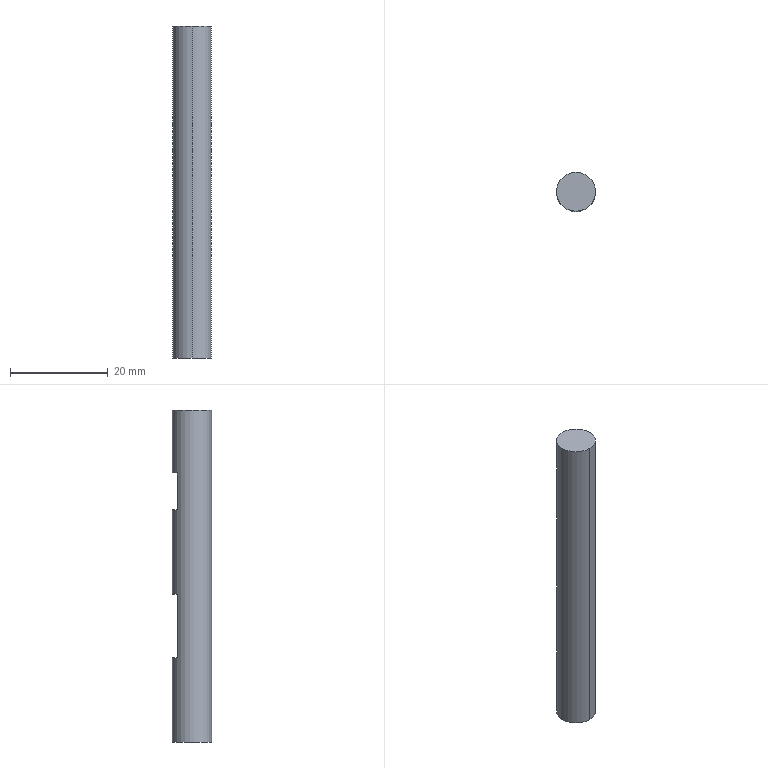Part | NX | 1 solid | 18 faces | box 8 x 8 x 68 mm | volume 3235 mm3 | plane 8 | cylinder 6 | cone 4 | commonest cylinder face diameters 3.3 x4 8 x2
STEP:
#1=CARTESIAN_POINT('',(-190.,200.7,-65.8));
#2=VERTEX_POINT('',#1);
#3=CARTESIAN_POINT('',(-190.,192.7,-65.8));
#4=VERTEX_POINT('',#3);
#5=CARTESIAN_POINT('',(-190.,196.7,-65.8));
#6=DIRECTION('',(0.,0.,1.));
#7=DIRECTION('',(0.,-1.,0.));
#8=AXIS2_PLACEMENT_3D('',#5,#6,#7);
#9=CIRCLE('',#8,4.);
#10=EDGE_CURVE('',#2,#4,#9,.T.);
#11=ORIENTED_EDGE('',*,*,#10,.T.);
#12=CARTESIAN_POINT('',(-190.,192.7,2.2));
#13=VERTEX_POINT('',#12);
#14=CARTESIAN_POINT('',(-190.,192.7,-55.8));
#15=DIRECTION('',(0.,0.,1.));
#16=VECTOR('',#15,1000.);
#17=LINE('',#14,#16);
#18=EDGE_CURVE('',#13,#4,#17,.F.);
#19=ORIENTED_EDGE('',*,*,#18,.F.);
#20=CARTESIAN_POINT('',(-190.,200.7,2.2));
#21=VERTEX_POINT('',#20);
#22=CARTESIAN_POINT('',(-190.,196.7,2.2));
#23=DIRECTION('',(0.,0.,1.));
#24=DIRECTION('',(0.,-1.,0.));
#25=AXIS2_PLACEMENT_3D('',#22,#23,#24);
#26=CIRCLE('',#25,4.);
#27=EDGE_CURVE('',#21,#13,#26,.T.);
#28=ORIENTED_EDGE('',*,*,#27,.F.);
#29=CARTESIAN_POINT('',(-190.,200.7,-10.7));
#30=VERTEX_POINT('',#29);
#31=CARTESIAN_POINT('',(-190.,200.7,-55.8));
#32=DIRECTION('',(0.,0.,1.));
#33=VECTOR('',#32,1000.);
#34=LINE('',#31,#33);
#35=EDGE_CURVE('',#30,#21,#34,.T.);
#36=ORIENTED_EDGE('',*,*,#35,.F.);
#37=CARTESIAN_POINT('',(-192.646,199.7,-10.7));
#38=VERTEX_POINT('',#37);
#39=CARTESIAN_POINT('',(-190.,196.7,-10.7));
#40=DIRECTION('',(0.,0.,1.));
#41=DIRECTION('',(0.,-1.,0.));
#42=AXIS2_PLACEMENT_3D('',#39,#40,#41);
#43=CIRCLE('',#42,4.);
#44=EDGE_CURVE('',#30,#38,#43,.T.);
#45=ORIENTED_EDGE('',*,*,#44,.T.);
#46=CARTESIAN_POINT('',(-192.646,199.7,-18.2));
#47=VERTEX_POINT('',#46);
#48=CARTESIAN_POINT('',(-192.646,199.7,-55.8));
#49=DIRECTION('',(0.,0.,1.));
#50=VECTOR('',#49,1000.);
#51=LINE('',#48,#50);
#52=EDGE_CURVE('',#47,#38,#51,.T.);
#53=ORIENTED_EDGE('',*,*,#52,.F.);
#54=CARTESIAN_POINT('',(-190.,200.7,-18.2));
#55=VERTEX_POINT('',#54);
#56=CARTESIAN_POINT('',(-190.,196.7,-18.2));
#57=DIRECTION('',(0.,0.,1.));
#58=DIRECTION('',(0.,-1.,0.));
#59=AXIS2_PLACEMENT_3D('',#56,#57,#58);
#60=CIRCLE('',#59,4.);
#61=EDGE_CURVE('',#55,#47,#60,.T.);
#62=ORIENTED_EDGE('',*,*,#61,.F.);
#63=CARTESIAN_POINT('',(-190.,200.7,-35.5));
#64=VERTEX_POINT('',#63);
#65=CARTESIAN_POINT('',(-190.,200.7,-55.8));
#66=DIRECTION('',(0.,0.,1.));
#67=VECTOR('',#66,1000.);
#68=LINE('',#65,#67);
#69=EDGE_CURVE('',#55,#64,#68,.F.);
#70=ORIENTED_EDGE('',*,*,#69,.T.);
#71=CARTESIAN_POINT('',(-192.646,199.7,-35.5));
#72=VERTEX_POINT('',#71);
#73=CARTESIAN_POINT('',(-190.,196.7,-35.5));
#74=DIRECTION('',(0.,0.,1.));
#75=DIRECTION('',(0.,-1.,0.));
#76=AXIS2_PLACEMENT_3D('',#73,#74,#75);
#77=CIRCLE('',#76,4.);
#78=EDGE_CURVE('',#64,#72,#77,.T.);
#79=ORIENTED_EDGE('',*,*,#78,.T.);
#80=CARTESIAN_POINT('',(-192.646,199.7,-48.5));
#81=VERTEX_POINT('',#80);
#82=CARTESIAN_POINT('',(-192.646,199.7,-55.8));
#83=DIRECTION('',(0.,0.,1.));
#84=VECTOR('',#83,1000.);
#85=LINE('',#82,#84);
#86=EDGE_CURVE('',#81,#72,#85,.T.);
#87=ORIENTED_EDGE('',*,*,#86,.F.);
#88=CARTESIAN_POINT('',(-190.,200.7,-48.5));
#89=VERTEX_POINT('',#88);
#90=CARTESIAN_POINT('',(-190.,196.7,-48.5));
#91=DIRECTION('',(0.,0.,1.));
#92=DIRECTION('',(0.,-1.,0.));
#93=AXIS2_PLACEMENT_3D('',#90,#91,#92);
#94=CIRCLE('',#93,4.);
#95=EDGE_CURVE('',#89,#81,#94,.T.);
#96=ORIENTED_EDGE('',*,*,#95,.F.);
#97=CARTESIAN_POINT('',(-190.,200.7,-55.8));
#98=DIRECTION('',(0.,0.,1.));
#99=VECTOR('',#98,1000.);
#100=LINE('',#97,#99);
#101=EDGE_CURVE('',#2,#89,#100,.T.);
#102=ORIENTED_EDGE('',*,*,#101,.F.);
#103=EDGE_LOOP('',(#11,#19,#28,#36,#45,#53,#62,#70,#79,#87,#96,#102));
#104=FACE_BOUND('',#103,.T.);
#105=CARTESIAN_POINT('',(-190.,196.7,-55.8));
#106=DIRECTION('',(0.,0.,1.));
#107=DIRECTION('',(0.,-1.,0.));
#108=AXIS2_PLACEMENT_3D('',#105,#106,#107);
#109=CYLINDRICAL_SURFACE('',#108,4.);
#110=ADVANCED_FACE('',(#104),#109,.T.);
#111=ORIENTED_EDGE('',*,*,#10,.F.);
#112=CARTESIAN_POINT('',(-190.,196.7,-65.8));
#113=DIRECTION('',(0.,0.,1.));
#114=DIRECTION('',(0.,-1.,0.));
#115=AXIS2_PLACEMENT_3D('',#112,#113,#114);
#116=CIRCLE('',#115,4.);
#117=EDGE_CURVE('',#4,#2,#116,.T.);
#118=ORIENTED_EDGE('',*,*,#117,.F.);
#119=EDGE_LOOP('',(#111,#118));
#120=FACE_BOUND('',#119,.T.);
#121=CARTESIAN_POINT('',(-187.685,196.7,-65.8));
#122=VERTEX_POINT('',#121);
#123=CARTESIAN_POINT('',(-192.315,196.7,-65.8));
#124=VERTEX_POINT('',#123);
#125=CARTESIAN_POINT('',(-190.,196.7,-65.8));
#126=DIRECTION('',(0.,0.,-1.));
#127=DIRECTION('',(-1.,0.,0.));
#128=AXIS2_PLACEMENT_3D('',#125,#126,#127);
#129=CIRCLE('',#128,2.315);
#130=EDGE_CURVE('',#122,#124,#129,.T.);
#131=ORIENTED_EDGE('',*,*,#130,.F.);
#132=CARTESIAN_POINT('',(-190.,196.7,-65.8));
#133=DIRECTION('',(0.,0.,-1.));
#134=DIRECTION('',(-1.,0.,0.));
#135=AXIS2_PLACEMENT_3D('',#132,#133,#134);
#136=CIRCLE('',#135,2.315);
#137=EDGE_CURVE('',#124,#122,#136,.T.);
#138=ORIENTED_EDGE('',*,*,#137,.F.);
#139=EDGE_LOOP('',(#131,#138));
#140=FACE_BOUND('',#139,.T.);
#141=CARTESIAN_POINT('',(-181.498,197.784,-65.8));
#142=DIRECTION('',(0.,0.,-1.));
#143=DIRECTION('',(-1.,0.,0.));
#144=AXIS2_PLACEMENT_3D('',#141,#142,#143);
#145=PLANE('',#144);
#146=ADVANCED_FACE('',(#120,#140),#145,.T.);
#147=ORIENTED_EDGE('',*,*,#27,.T.);
#148=CARTESIAN_POINT('',(-190.,196.7,2.2));
#149=DIRECTION('',(0.,0.,1.));
#150=DIRECTION('',(0.,-1.,0.));
#151=AXIS2_PLACEMENT_3D('',#148,#149,#150);
#152=CIRCLE('',#151,4.);
#153=EDGE_CURVE('',#13,#21,#152,.T.);
#154=ORIENTED_EDGE('',*,*,#153,.T.);
#155=EDGE_LOOP('',(#147,#154));
#156=FACE_BOUND('',#155,.T.);
#157=CARTESIAN_POINT('',(-181.498,197.784,2.2));
#158=DIRECTION('',(0.,0.,-1.));
#159=DIRECTION('',(-1.,0.,0.));
#160=AXIS2_PLACEMENT_3D('',#157,#158,#159);
#161=PLANE('',#160);
#162=ADVANCED_FACE('',(#156),#161,.F.);
#163=CARTESIAN_POINT('',(-187.354,199.7,-48.5));
#164=VERTEX_POINT('',#163);
#165=CARTESIAN_POINT('',(-187.354,199.7,-35.5));
#166=VERTEX_POINT('',#165);
#167=CARTESIAN_POINT('',(-187.354,199.7,-55.8));
#168=DIRECTION('',(0.,0.,1.));
#169=VECTOR('',#168,1000.);
#170=LINE('',#167,#169);
#171=EDGE_CURVE('',#164,#166,#170,.T.);
#172=ORIENTED_EDGE('',*,*,#171,.F.);
#173=CARTESIAN_POINT('',(-190.,199.7,-48.5));
#174=DIRECTION('',(1.,0.,0.));
#175=VECTOR('',#174,1000.);
#176=LINE('',#173,#175);
#177=EDGE_CURVE('',#81,#164,#176,.T.);
#178=ORIENTED_EDGE('',*,*,#177,.F.);
#179=ORIENTED_EDGE('',*,*,#86,.T.);
#180=CARTESIAN_POINT('',(-190.,199.7,-35.5));
#181=DIRECTION('',(1.,0.,0.));
#182=VECTOR('',#181,1000.);
#183=LINE('',#180,#182);
#184=EDGE_CURVE('',#72,#166,#183,.T.);
#185=ORIENTED_EDGE('',*,*,#184,.T.);
#186=EDGE_LOOP('',(#172,#178,#179,#185));
#187=FACE_BOUND('',#186,.T.);
#188=CARTESIAN_POINT('',(-169.84,199.7,-22.748));
#189=DIRECTION('',(0.,1.,0.));
#190=DIRECTION('',(1.,0.,0.));
#191=AXIS2_PLACEMENT_3D('',#188,#189,#190);
#192=PLANE('',#191);
#193=ADVANCED_FACE('',(#187),#192,.T.);
#194=CARTESIAN_POINT('',(-187.354,199.7,-18.2));
#195=VERTEX_POINT('',#194);
#196=CARTESIAN_POINT('',(-190.,199.7,-18.2));
#197=DIRECTION('',(1.,0.,0.));
#198=VECTOR('',#197,1000.);
#199=LINE('',#196,#198);
#200=EDGE_CURVE('',#47,#195,#199,.T.);
#201=ORIENTED_EDGE('',*,*,#200,.T.);
#202=CARTESIAN_POINT('',(-190.,196.7,-18.2));
#203=DIRECTION('',(0.,0.,1.));
#204=DIRECTION('',(0.,-1.,0.));
#205=AXIS2_PLACEMENT_3D('',#202,#203,#204);
#206=CIRCLE('',#205,4.);
#207=EDGE_CURVE('',#195,#55,#206,.T.);
#208=ORIENTED_EDGE('',*,*,#207,.T.);
#209=ORIENTED_EDGE('',*,*,#61,.T.);
#210=EDGE_LOOP('',(#201,#208,#209));
#211=FACE_BOUND('',#210,.T.);
#212=CARTESIAN_POINT('',(-185.645,200.992,-18.2));
#213=DIRECTION('',(0.,0.,1.));
#214=DIRECTION('',(1.,0.,0.));
#215=AXIS2_PLACEMENT_3D('',#212,#213,#214);
#216=PLANE('',#215);
#217=ADVANCED_FACE('',(#211),#216,.T.);
#218=CARTESIAN_POINT('',(-187.354,199.7,-10.7));
#219=VERTEX_POINT('',#218);
#220=CARTESIAN_POINT('',(-187.354,199.7,-55.8));
#221=DIRECTION('',(0.,0.,1.));
#222=VECTOR('',#221,1000.);
#223=LINE('',#220,#222);
#224=EDGE_CURVE('',#195,#219,#223,.T.);
#225=ORIENTED_EDGE('',*,*,#224,.F.);
#226=ORIENTED_EDGE('',*,*,#200,.F.);
#227=ORIENTED_EDGE('',*,*,#52,.T.);
#228=CARTESIAN_POINT('',(-181.498,199.7,-10.7));
#229=DIRECTION('',(-1.,0.,0.));
#230=VECTOR('',#229,1000.);
#231=LINE('',#228,#230);
#232=EDGE_CURVE('',#219,#38,#231,.T.);
#233=ORIENTED_EDGE('',*,*,#232,.F.);
#234=EDGE_LOOP('',(#225,#226,#227,#233));
#235=FACE_BOUND('',#234,.T.);
#236=CARTESIAN_POINT('',(-192.646,199.7,-13.2));
#237=DIRECTION('',(0.,-1.,0.));
#238=DIRECTION('',(-1.,0.,0.));
#239=AXIS2_PLACEMENT_3D('',#236,#237,#238);
#240=PLANE('',#239);
#241=ADVANCED_FACE('',(#235),#240,.F.);
#242=ORIENTED_EDGE('',*,*,#44,.F.);
#243=CARTESIAN_POINT('',(-190.,196.7,-10.7));
#244=DIRECTION('',(0.,0.,1.));
#245=DIRECTION('',(0.,-1.,0.));
#246=AXIS2_PLACEMENT_3D('',#243,#244,#245);
#247=CIRCLE('',#246,4.);
#248=EDGE_CURVE('',#219,#30,#247,.T.);
#249=ORIENTED_EDGE('',*,*,#248,.F.);
#250=ORIENTED_EDGE('',*,*,#232,.T.);
#251=EDGE_LOOP('',(#242,#249,#250));
#252=FACE_BOUND('',#251,.T.);
#253=CARTESIAN_POINT('',(-185.645,200.992,-10.7));
#254=DIRECTION('',(0.,0.,1.));
#255=DIRECTION('',(1.,0.,0.));
#256=AXIS2_PLACEMENT_3D('',#253,#254,#255);
#257=PLANE('',#256);
#258=ADVANCED_FACE('',(#252),#257,.F.);
#259=ORIENTED_EDGE('',*,*,#95,.T.);
#260=ORIENTED_EDGE('',*,*,#177,.T.);
#261=CARTESIAN_POINT('',(-190.,196.7,-48.5));
#262=DIRECTION('',(0.,0.,1.));
#263=DIRECTION('',(0.,-1.,0.));
#264=AXIS2_PLACEMENT_3D('',#261,#262,#263);
#265=CIRCLE('',#264,4.);
#266=EDGE_CURVE('',#164,#89,#265,.T.);
#267=ORIENTED_EDGE('',*,*,#266,.T.);
#268=EDGE_LOOP('',(#259,#260,#267));
#269=FACE_BOUND('',#268,.T.);
#270=CARTESIAN_POINT('',(-190.,214.7,-48.5));
#271=DIRECTION('',(0.,0.,-1.));
#272=DIRECTION('',(-1.,0.,0.));
#273=AXIS2_PLACEMENT_3D('',#270,#271,#272);
#274=PLANE('',#273);
#275=ADVANCED_FACE('',(#269),#274,.F.);
#276=ORIENTED_EDGE('',*,*,#78,.F.);
#277=CARTESIAN_POINT('',(-190.,196.7,-35.5));
#278=DIRECTION('',(0.,0.,1.));
#279=DIRECTION('',(0.,-1.,0.));
#280=AXIS2_PLACEMENT_3D('',#277,#278,#279);
#281=CIRCLE('',#280,4.);
#282=EDGE_CURVE('',#166,#64,#281,.T.);
#283=ORIENTED_EDGE('',*,*,#282,.F.);
#284=ORIENTED_EDGE('',*,*,#184,.F.);
#285=EDGE_LOOP('',(#276,#283,#284));
#286=FACE_BOUND('',#285,.T.);
#287=CARTESIAN_POINT('',(-190.,214.7,-35.5));
#288=DIRECTION('',(0.,0.,1.));
#289=DIRECTION('',(1.,0.,0.));
#290=AXIS2_PLACEMENT_3D('',#287,#288,#289);
#291=PLANE('',#290);
#292=ADVANCED_FACE('',(#286),#291,.F.);
#293=CARTESIAN_POINT('',(-188.35,196.7,-65.416));
#294=VERTEX_POINT('',#293);
#295=CARTESIAN_POINT('',(-191.65,196.7,-65.416));
#296=VERTEX_POINT('',#295);
#297=CARTESIAN_POINT('',(-190.,196.7,-65.416));
#298=DIRECTION('',(0.,0.,-1.));
#299=DIRECTION('',(-1.,0.,0.));
#300=AXIS2_PLACEMENT_3D('',#297,#298,#299);
#301=CIRCLE('',#300,1.65);
#302=EDGE_CURVE('',#294,#296,#301,.T.);
#303=ORIENTED_EDGE('',*,*,#302,.T.);
#304=CARTESIAN_POINT('',(-191.65,196.7,-57.8));
#305=VERTEX_POINT('',#304);
#306=CARTESIAN_POINT('',(-191.65,196.7,-65.8));
#307=DIRECTION('',(0.,0.,-1.));
#308=VECTOR('',#307,1000.);
#309=LINE('',#306,#308);
#310=EDGE_CURVE('',#296,#305,#309,.F.);
#311=ORIENTED_EDGE('',*,*,#310,.T.);
#312=CARTESIAN_POINT('',(-188.35,196.7,-57.8));
#313=VERTEX_POINT('',#312);
#314=CARTESIAN_POINT('',(-190.,196.7,-57.8));
#315=DIRECTION('',(0.,0.,-1.));
#316=DIRECTION('',(-1.,0.,0.));
#317=AXIS2_PLACEMENT_3D('',#314,#315,#316);
#318=CIRCLE('',#317,1.65);
#319=EDGE_CURVE('',#313,#305,#318,.T.);
#320=ORIENTED_EDGE('',*,*,#319,.F.);
#321=CARTESIAN_POINT('',(-188.35,196.7,-65.8));
#322=DIRECTION('',(0.,0.,-1.));
#323=VECTOR('',#322,1000.);
#324=LINE('',#321,#323);
#325=EDGE_CURVE('',#294,#313,#324,.F.);
#326=ORIENTED_EDGE('',*,*,#325,.F.);
#327=EDGE_LOOP('',(#303,#311,#320,#326));
#328=FACE_BOUND('',#327,.T.);
#329=CARTESIAN_POINT('',(-190.,196.7,-65.8));
#330=DIRECTION('',(0.,0.,-1.));
#331=DIRECTION('',(-1.,0.,0.));
#332=AXIS2_PLACEMENT_3D('',#329,#330,#331);
#333=CYLINDRICAL_SURFACE('',#332,1.65);
#334=ADVANCED_FACE('',(#328),#333,.F.);
#335=ORIENTED_EDGE('',*,*,#319,.T.);
#336=CARTESIAN_POINT('',(-191.65,196.7,-53.6));
#337=VERTEX_POINT('',#336);
#338=CARTESIAN_POINT('',(-191.65,196.7,-65.8));
#339=DIRECTION('',(0.,0.,-1.));
#340=VECTOR('',#339,1000.);
#341=LINE('',#338,#340);
#342=EDGE_CURVE('',#305,#337,#341,.F.);
#343=ORIENTED_EDGE('',*,*,#342,.T.);
#344=CARTESIAN_POINT('',(-188.35,196.7,-53.6));
#345=VERTEX_POINT('',#344);
#346=CARTESIAN_POINT('',(-190.,196.7,-53.6));
#347=DIRECTION('',(0.,0.,-1.));
#348=DIRECTION('',(-1.,0.,0.));
#349=AXIS2_PLACEMENT_3D('',#346,#347,#348);
#350=CIRCLE('',#349,1.65);
#351=EDGE_CURVE('',#345,#337,#350,.T.);
#352=ORIENTED_EDGE('',*,*,#351,.F.);
#353=CARTESIAN_POINT('',(-188.35,196.7,-65.8));
#354=DIRECTION('',(0.,0.,-1.));
#355=VECTOR('',#354,1000.);
#356=LINE('',#353,#355);
#357=EDGE_CURVE('',#313,#345,#356,.F.);
#358=ORIENTED_EDGE('',*,*,#357,.F.);
#359=EDGE_LOOP('',(#335,#343,#352,#358));
#360=FACE_BOUND('',#359,.T.);
#361=CARTESIAN_POINT('',(-190.,196.7,-65.8));
#362=DIRECTION('',(0.,0.,-1.));
#363=DIRECTION('',(-1.,0.,0.));
#364=AXIS2_PLACEMENT_3D('',#361,#362,#363);
#365=CYLINDRICAL_SURFACE('',#364,1.65);
#366=ADVANCED_FACE('',(#360),#365,.F.);
#367=ORIENTED_EDGE('',*,*,#351,.T.);
#368=CARTESIAN_POINT('',(-190.,196.7,-52.609));
#369=VERTEX_POINT('',#368);
#370=CARTESIAN_POINT('',(-191.65,196.7,-53.6));
#371=DIRECTION('',(-0.8572,0.,-0.515));
#372=VECTOR('',#371,1000.);
#373=LINE('',#370,#372);
#374=EDGE_CURVE('',#369,#337,#373,.T.);
#375=ORIENTED_EDGE('',*,*,#374,.F.);
#376=CARTESIAN_POINT('',(-188.35,196.7,-53.6));
#377=DIRECTION('',(0.8572,0.,-0.515));
#378=VECTOR('',#377,1000.);
#379=LINE('',#376,#378);
#380=EDGE_CURVE('',#369,#345,#379,.T.);
#381=ORIENTED_EDGE('',*,*,#380,.T.);
#382=EDGE_LOOP('',(#367,#375,#381));
#383=FACE_BOUND('',#382,.T.);
#384=CARTESIAN_POINT('',(-190.,196.7,-53.6));
#385=DIRECTION('',(0.,0.,-1.));
#386=DIRECTION('',(-1.,0.,0.));
#387=AXIS2_PLACEMENT_3D('',#384,#385,#386);
#388=CONICAL_SURFACE('',#387,1.65,1.03);
#389=ADVANCED_FACE('',(#383),#388,.F.);
#390=ORIENTED_EDGE('',*,*,#302,.F.);
#391=CARTESIAN_POINT('',(-188.35,196.7,-65.416));
#392=DIRECTION('',(0.866,0.,-0.5));
#393=VECTOR('',#392,1000.);
#394=LINE('',#391,#393);
#395=EDGE_CURVE('',#122,#294,#394,.F.);
#396=ORIENTED_EDGE('',*,*,#395,.F.);
#397=ORIENTED_EDGE('',*,*,#130,.T.);
#398=CARTESIAN_POINT('',(-191.65,196.7,-65.416));
#399=DIRECTION('',(-0.866,0.,-0.5));
#400=VECTOR('',#399,1000.);
#401=LINE('',#398,#400);
#402=EDGE_CURVE('',#124,#296,#401,.F.);
#403=ORIENTED_EDGE('',*,*,#402,.T.);
#404=EDGE_LOOP('',(#390,#396,#397,#403));
#405=FACE_BOUND('',#404,.T.);
#406=CARTESIAN_POINT('',(-190.,196.7,-65.416));
#407=DIRECTION('',(0.,0.,-1.));
#408=DIRECTION('',(-1.,0.,0.));
#409=AXIS2_PLACEMENT_3D('',#406,#407,#408);
#410=CONICAL_SURFACE('',#409,1.65,1.047);
#411=ADVANCED_FACE('',(#405),#410,.F.);
#412=ORIENTED_EDGE('',*,*,#402,.F.);
#413=ORIENTED_EDGE('',*,*,#137,.T.);
#414=ORIENTED_EDGE('',*,*,#395,.T.);
#415=CARTESIAN_POINT('',(-190.,196.7,-65.416));
#416=DIRECTION('',(0.,0.,-1.));
#417=DIRECTION('',(-1.,0.,0.));
#418=AXIS2_PLACEMENT_3D('',#415,#416,#417);
#419=CIRCLE('',#418,1.65);
#420=EDGE_CURVE('',#296,#294,#419,.T.);
#421=ORIENTED_EDGE('',*,*,#420,.F.);
#422=EDGE_LOOP('',(#412,#413,#414,#421));
#423=FACE_BOUND('',#422,.T.);
#424=CARTESIAN_POINT('',(-190.,196.7,-65.416));
#425=DIRECTION('',(0.,0.,-1.));
#426=DIRECTION('',(-1.,0.,0.));
#427=AXIS2_PLACEMENT_3D('',#424,#425,#426);
#428=CONICAL_SURFACE('',#427,1.65,1.047);
#429=ADVANCED_FACE('',(#423),#428,.F.);
#430=ORIENTED_EDGE('',*,*,#35,.T.);
#431=ORIENTED_EDGE('',*,*,#153,.F.);
#432=ORIENTED_EDGE('',*,*,#18,.T.);
#433=ORIENTED_EDGE('',*,*,#117,.T.);
#434=ORIENTED_EDGE('',*,*,#101,.T.);
#435=ORIENTED_EDGE('',*,*,#266,.F.);
#436=ORIENTED_EDGE('',*,*,#171,.T.);
#437=ORIENTED_EDGE('',*,*,#282,.T.);
#438=ORIENTED_EDGE('',*,*,#69,.F.);
#439=ORIENTED_EDGE('',*,*,#207,.F.);
#440=ORIENTED_EDGE('',*,*,#224,.T.);
#441=ORIENTED_EDGE('',*,*,#248,.T.);
#442=EDGE_LOOP('',(#430,#431,#432,#433,#434,#435,#436,#437,#438,#439,#440,#441));
#443=FACE_BOUND('',#442,.T.);
#444=CARTESIAN_POINT('',(-190.,196.7,-55.8));
#445=DIRECTION('',(0.,0.,1.));
#446=DIRECTION('',(0.,-1.,0.));
#447=AXIS2_PLACEMENT_3D('',#444,#445,#446);
#448=CYLINDRICAL_SURFACE('',#447,4.);
#449=ADVANCED_FACE('',(#443),#448,.T.);
#450=ORIENTED_EDGE('',*,*,#380,.F.);
#451=ORIENTED_EDGE('',*,*,#374,.T.);
#452=CARTESIAN_POINT('',(-190.,196.7,-53.6));
#453=DIRECTION('',(0.,0.,-1.));
#454=DIRECTION('',(-1.,0.,0.));
#455=AXIS2_PLACEMENT_3D('',#452,#453,#454);
#456=CIRCLE('',#455,1.65);
#457=EDGE_CURVE('',#337,#345,#456,.T.);
#458=ORIENTED_EDGE('',*,*,#457,.T.);
#459=EDGE_LOOP('',(#450,#451,#458));
#460=FACE_BOUND('',#459,.T.);
#461=CARTESIAN_POINT('',(-190.,196.7,-53.6));
#462=DIRECTION('',(0.,0.,-1.));
#463=DIRECTION('',(-1.,0.,0.));
#464=AXIS2_PLACEMENT_3D('',#461,#462,#463);
#465=CONICAL_SURFACE('',#464,1.65,1.03);
#466=ADVANCED_FACE('',(#460),#465,.F.);
#467=ORIENTED_EDGE('',*,*,#342,.F.);
#468=CARTESIAN_POINT('',(-190.,196.7,-57.8));
#469=DIRECTION('',(0.,0.,-1.));
#470=DIRECTION('',(-1.,0.,0.));
#471=AXIS2_PLACEMENT_3D('',#468,#469,#470);
#472=CIRCLE('',#471,1.65);
#473=EDGE_CURVE('',#305,#313,#472,.T.);
#474=ORIENTED_EDGE('',*,*,#473,.T.);
#475=ORIENTED_EDGE('',*,*,#357,.T.);
#476=ORIENTED_EDGE('',*,*,#457,.F.);
#477=EDGE_LOOP('',(#467,#474,#475,#476));
#478=FACE_BOUND('',#477,.T.);
#479=CARTESIAN_POINT('',(-190.,196.7,-65.8));
#480=DIRECTION('',(0.,0.,-1.));
#481=DIRECTION('',(-1.,0.,0.));
#482=AXIS2_PLACEMENT_3D('',#479,#480,#481);
#483=CYLINDRICAL_SURFACE('',#482,1.65);
#484=ADVANCED_FACE('',(#478),#483,.F.);
#485=ORIENTED_EDGE('',*,*,#310,.F.);
#486=ORIENTED_EDGE('',*,*,#420,.T.);
#487=ORIENTED_EDGE('',*,*,#325,.T.);
#488=ORIENTED_EDGE('',*,*,#473,.F.);
#489=EDGE_LOOP('',(#485,#486,#487,#488));
#490=FACE_BOUND('',#489,.T.);
#491=CARTESIAN_POINT('',(-190.,196.7,-65.8));
#492=DIRECTION('',(0.,0.,-1.));
#493=DIRECTION('',(-1.,0.,0.));
#494=AXIS2_PLACEMENT_3D('',#491,#492,#493);
#495=CYLINDRICAL_SURFACE('',#494,1.65);
#496=ADVANCED_FACE('',(#490),#495,.F.);
#497=CLOSED_SHELL('',(#110,#146,#162,#193,#217,#241,#258,#275,#292,#334,#366,#389,#411,#429,#449,#466,#484,#496));
#498=MANIFOLD_SOLID_BREP('',#497);
#499=(LENGTH_UNIT()NAMED_UNIT(*)SI_UNIT(.MILLI.,.METRE.));
#500=UNCERTAINTY_MEASURE_WITH_UNIT(LENGTH_MEASURE(0.00001),#499,'','');
#501=(NAMED_UNIT(*)PLANE_ANGLE_UNIT()SI_UNIT($,.RADIAN.));
#502=(NAMED_UNIT(*)SI_UNIT($,.STERADIAN.)SOLID_ANGLE_UNIT());
#503=(GEOMETRIC_REPRESENTATION_CONTEXT(3)GLOBAL_UNCERTAINTY_ASSIGNED_CONTEXT((#500))GLOBAL_UNIT_ASSIGNED_CONTEXT((#499,#501,#502))REPRESENTATION_CONTEXT('',''));
#504=ADVANCED_BREP_SHAPE_REPRESENTATION('',(#498),#503);